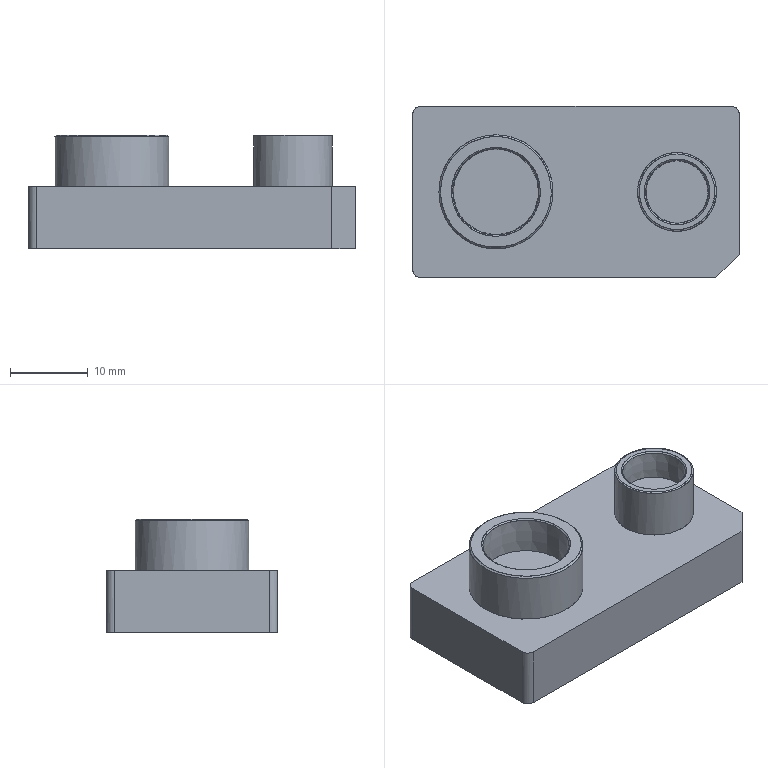NC program | PowerMill | posted by the shop | part box 42 x 22 x 14.621 mm
Lines 4390 to 5888 of 126517:
( TOOL ID   D4C_1_1 )
( TOOL DIA. 4. TIP RAD 0 LENGTH 61.8 )
( Z = -6.75 )
T2 M6
T3
G91 G28 Z0
G0 G90 G54
M08
S18000 M3
X0 Y0 M8
G43 Z9.801 H2
X-19.073 Y-5.404
Z.797
G1 Z-.403 F3600
X-19.051 Y-5.405 F6000
G3 X-18.846 Y-5.215 I.008 J.198
G1 X-18.79 Y-3.832
X-19.034 Y-3.291
X-19.237 Y-2.684
X-19.48 Y-1.708
X-19.605 Y-.732
X-19.627 Y.244
X-19.557 Y1.22
X-19.373 Y2.196
X-19.034 Y3.291
X-18.546 Y4.373
X-18.058 Y5.183
X-17.756 Y5.613
X-17.082 Y6.417
X-16.594 Y6.892
X-15.772 Y7.565
X-15.13 Y7.982
X-14.642 Y8.259
X-14.154 Y8.499
X-13.665 Y8.706
X-13.177 Y8.88
X-12.689 Y9.023
X-11.713 Y9.218
X-10.737 Y9.319
X-9.761 Y9.318
X-8.785 Y9.201
X-7.94 Y9.029
X-7.321 Y8.842
X-6.833 Y8.664
X-6.345 Y8.452
X-5.601 Y8.053
X-4.837 Y7.565
X-4.392 Y7.222
X-3.904 Y6.794
X-3.416 Y6.294
X-2.853 Y5.613
X-2.44 Y5.027
X-1.952 Y4.152
X-1.727 Y3.66
X-1.464 Y2.987
X-1.372 Y2.684
X-1.129 Y1.708
X-1.004 Y.732
X-.982 Y-.244
X-1.051 Y-1.22
X-1.236 Y-2.196
X-1.464 Y-2.987
X-1.727 Y-3.66
X-1.95 Y-4.148
X-2.44 Y-5.027
X-2.853 Y-5.613
X-3.249 Y-6.101
X-3.904 Y-6.794
X-4.392 Y-7.222
X-4.837 Y-7.565
X-5.369 Y-7.921
X-5.857 Y-8.205
X-6.561 Y-8.541
X-7.321 Y-8.842
X-7.94 Y-9.029
X-8.785 Y-9.201
X-9.761 Y-9.318
X-10.737 Y-9.319
X-11.713 Y-9.218
X-12.668 Y-9.029
X-13.177 Y-8.88
X-14.048 Y-8.541
X-14.642 Y-8.259
X-15.13 Y-7.982
X-15.772 Y-7.565
X-16.382 Y-7.077
X-17.082 Y-6.417
X-17.57 Y-5.855
X-18.1 Y-5.125
X-18.546 Y-4.373
X-18.79 Y-3.832
X-19.073 Y-5.408 Z-.596
X-19.051 Y-5.409
G3 X-18.846 Y-5.219 I.008 J.198
G1 X-18.79 Y-3.832
X-19.034 Y-3.291
X-19.237 Y-2.684
X-19.48 Y-1.708
X-19.605 Y-.732
X-19.627 Y.244
X-19.557 Y1.22
X-19.373 Y2.196
X-19.034 Y3.291
X-18.546 Y4.373
X-18.058 Y5.183
X-17.756 Y5.613
X-17.082 Y6.417
X-16.594 Y6.892
X-15.772 Y7.565
X-15.13 Y7.982
X-14.642 Y8.259
X-14.154 Y8.499
X-13.665 Y8.706
X-13.177 Y8.88
X-12.689 Y9.023
X-11.713 Y9.218
X-10.737 Y9.319
X-9.761 Y9.318
X-8.785 Y9.201
X-7.94 Y9.029
X-7.321 Y8.842
X-6.833 Y8.664
X-6.345 Y8.452
X-5.601 Y8.053
X-4.837 Y7.565
X-4.392 Y7.222
X-3.904 Y6.794
X-3.416 Y6.294
X-2.853 Y5.613
X-2.44 Y5.027
X-1.952 Y4.152
X-1.727 Y3.66
X-1.464 Y2.987
X-1.372 Y2.684
X-1.129 Y1.708
X-1.004 Y.732
X-.982 Y-.244
X-1.051 Y-1.22
X-1.236 Y-2.196
X-1.464 Y-2.987
X-1.727 Y-3.66
X-1.95 Y-4.148
X-2.44 Y-5.027
X-2.853 Y-5.613
X-3.249 Y-6.101
X-3.904 Y-6.794
X-4.392 Y-7.222
X-4.837 Y-7.565
X-5.369 Y-7.921
X-5.857 Y-8.205
X-6.561 Y-8.541
X-7.321 Y-8.842
X-7.94 Y-9.029
X-8.785 Y-9.201
X-9.761 Y-9.318
X-10.737 Y-9.319
X-11.713 Y-9.218
X-12.668 Y-9.029
X-13.177 Y-8.88
X-14.048 Y-8.541
X-14.642 Y-8.259
X-15.13 Y-7.982
X-15.772 Y-7.565
X-16.382 Y-7.077
X-17.082 Y-6.417
X-17.57 Y-5.855
X-18.1 Y-5.125
X-18.546 Y-4.373
X-18.79 Y-3.832
X-19.073 Y-5.408 Z-.79
X-19.051 Y-5.409
G3 X-18.846 Y-5.219 I.008 J.198
G1 X-18.79 Y-3.832
X-19.034 Y-3.291
X-19.237 Y-2.684
X-19.48 Y-1.708
X-19.605 Y-.732
X-19.627 Y.244
X-19.557 Y1.22
X-19.373 Y2.196
X-19.034 Y3.291
X-18.546 Y4.373
X-18.058 Y5.183
X-17.756 Y5.613
X-17.082 Y6.417
X-16.594 Y6.892
X-15.772 Y7.565
X-15.13 Y7.982
X-14.642 Y8.259
X-14.154 Y8.499
X-13.665 Y8.706
X-13.177 Y8.88
X-12.689 Y9.023
X-11.713 Y9.218
X-10.737 Y9.319
X-9.761 Y9.318
X-8.785 Y9.201
X-7.94 Y9.029
X-7.321 Y8.842
X-6.833 Y8.664
X-6.345 Y8.452
X-5.601 Y8.053
X-4.837 Y7.565
X-4.392 Y7.222
X-3.904 Y6.794
X-3.416 Y6.294
X-2.853 Y5.613
X-2.44 Y5.027
X-2.129 Y4.468
X-1.952 Y4.152
X-1.95 Y4.148
X-1.727 Y3.66
X-1.464 Y2.987
X-1.372 Y2.684
X-1.129 Y1.708
X-1.004 Y.732
X-.982 Y-.244
X-1.051 Y-1.22
X-1.236 Y-2.196
X-1.464 Y-2.987
X-1.727 Y-3.66
X-1.779 Y-3.773
X-1.95 Y-4.148
X-1.952 Y-4.15
Y-4.152
X-2.44 Y-5.027
X-2.853 Y-5.613
X-3.249 Y-6.101
X-3.904 Y-6.794
X-4.392 Y-7.222
X-4.837 Y-7.565
X-5.369 Y-7.921
X-5.857 Y-8.205
X-6.561 Y-8.541
X-7.321 Y-8.842
X-7.94 Y-9.029
X-8.785 Y-9.201
X-9.761 Y-9.318
X-10.737 Y-9.319
X-11.713 Y-9.218
X-12.668 Y-9.029
X-13.177 Y-8.88
X-14.048 Y-8.541
X-14.642 Y-8.259
X-15.13 Y-7.982
X-15.772 Y-7.565
X-16.382 Y-7.077
X-17.082 Y-6.417
X-17.57 Y-5.855
X-18.1 Y-5.125
X-18.546 Y-4.373
X-18.79 Y-3.832
X-19.073 Y-5.408 Z-.984
X-19.051 Y-5.409
G3 X-18.846 Y-5.219 I.008 J.198
G1 X-18.79 Y-3.832
X-19.034 Y-3.291
X-19.237 Y-2.684
X-19.48 Y-1.708
X-19.605 Y-.732
X-19.627 Y.244
X-19.558 Y1.22
X-19.373 Y2.196
X-19.034 Y3.291
X-18.546 Y4.373
X-18.058 Y5.183
X-17.756 Y5.613
X-17.082 Y6.417
X-16.594 Y6.892
X-15.772 Y7.565
X-15.13 Y7.982
X-14.642 Y8.259
X-14.154 Y8.499
X-13.665 Y8.706
X-13.177 Y8.88
X-12.689 Y9.023
X-11.713 Y9.218
X-10.737 Y9.319
X-9.761 Y9.318
X-8.785 Y9.201
X-7.94 Y9.029
X-7.321 Y8.842
X-6.833 Y8.664
X-6.345 Y8.452
X-5.601 Y8.053
X-4.837 Y7.565
X-4.392 Y7.222
X-3.904 Y6.794
X-3.416 Y6.294
X-2.853 Y5.613
X-2.44 Y5.027
X-1.95 Y4.148
X-1.727 Y3.66
X-1.464 Y2.987
X-1.372 Y2.684
X-1.129 Y1.708
X-1.004 Y.732
X-.982 Y-.244
X-1.051 Y-1.22
X-1.236 Y-2.196
X-1.464 Y-2.987
X-1.727 Y-3.66
X-1.83 Y-3.884
X-1.95 Y-4.148
X-1.951 Y-4.15
X-1.952 Y-4.152
X-2.44 Y-5.027
X-2.853 Y-5.613
X-3.249 Y-6.101
X-3.904 Y-6.794
X-4.392 Y-7.222
X-4.837 Y-7.565
X-5.369 Y-7.921
X-5.857 Y-8.205
X-6.561 Y-8.541
X-7.321 Y-8.842
X-7.94 Y-9.029
X-8.785 Y-9.201
X-9.761 Y-9.318
X-10.737 Y-9.319
X-11.713 Y-9.218
X-12.668 Y-9.029
X-13.177 Y-8.88
X-14.048 Y-8.541
X-14.642 Y-8.259
X-15.13 Y-7.982
X-15.772 Y-7.565
X-16.382 Y-7.077
X-17.082 Y-6.417
X-17.57 Y-5.855
X-18.1 Y-5.125
X-18.546 Y-4.373
X-18.79 Y-3.832
X-19.073 Y-5.408 Z-1.177
X-19.051 Y-5.409
G3 X-18.846 Y-5.219 I.008 J.198
G1 X-18.79 Y-3.832
X-19.034 Y-3.291
X-19.237 Y-2.684
X-19.48 Y-1.708
X-19.605 Y-.732
X-19.627 Y.244
X-19.558 Y1.22
X-19.373 Y2.196
X-19.034 Y3.291
X-18.546 Y4.373
X-18.058 Y5.183
X-17.756 Y5.613
X-17.082 Y6.417
X-16.594 Y6.892
X-15.772 Y7.565
X-15.13 Y7.982
X-14.642 Y8.259
X-14.154 Y8.499
X-13.665 Y8.706
X-13.177 Y8.88
X-12.689 Y9.023
X-11.713 Y9.218
X-10.737 Y9.319
X-9.761 Y9.318
X-8.785 Y9.201
X-7.94 Y9.029
X-7.321 Y8.842
X-6.833 Y8.664
X-6.345 Y8.452
X-5.601 Y8.053
X-4.837 Y7.565
X-4.392 Y7.222
X-3.904 Y6.794
X-3.416 Y6.294
X-2.853 Y5.613
X-2.44 Y5.027
X-1.95 Y4.148
X-1.727 Y3.66
X-1.464 Y2.987
X-1.372 Y2.684
X-1.129 Y1.708
X-1.004 Y.732
X-.982 Y-.244
X-1.051 Y-1.22
X-1.236 Y-2.196
X-1.464 Y-2.987
X-1.727 Y-3.66
X-1.88 Y-3.993
X-1.951 Y-4.148
Y-4.15
X-1.952 Y-4.152
X-2.44 Y-5.027
X-2.853 Y-5.613
X-3.249 Y-6.101
X-3.904 Y-6.794
X-4.392 Y-7.222
X-4.837 Y-7.565
X-5.369 Y-7.921
X-5.857 Y-8.205
X-6.561 Y-8.541
X-7.321 Y-8.842
X-7.94 Y-9.029
X-8.785 Y-9.201
X-9.761 Y-9.318
X-10.737 Y-9.319
X-11.713 Y-9.218
X-12.668 Y-9.029
X-13.177 Y-8.88
X-14.048 Y-8.541
X-14.642 Y-8.259
X-15.13 Y-7.982
X-15.772 Y-7.565
X-16.382 Y-7.077
X-17.082 Y-6.417
X-17.57 Y-5.855
X-18.1 Y-5.125
X-18.546 Y-4.373
X-18.79 Y-3.832
X-19.073 Y-5.408 Z-1.371
X-19.051 Y-5.409
G3 X-18.846 Y-5.219 I.008 J.198
G1 X-18.79 Y-3.832
X-19.034 Y-3.291
X-19.237 Y-2.684
X-19.48 Y-1.708
X-19.605 Y-.732
X-19.627 Y.244
X-19.558 Y1.22
X-19.373 Y2.196
X-19.034 Y3.291
X-18.546 Y4.373
X-18.058 Y5.183
X-17.756 Y5.613
X-17.082 Y6.417
X-16.594 Y6.892
X-15.772 Y7.565
X-15.13 Y7.982
X-14.642 Y8.259
X-14.154 Y8.499
X-13.665 Y8.706
X-13.177 Y8.88
X-12.689 Y9.023
X-11.713 Y9.218
X-10.737 Y9.319
X-9.761 Y9.318
X-8.785 Y9.201
X-7.94 Y9.029
X-7.321 Y8.842
X-6.833 Y8.664
X-6.345 Y8.452
X-5.601 Y8.053
X-4.837 Y7.565
X-4.392 Y7.222
X-3.904 Y6.794
X-3.416 Y6.294
X-2.853 Y5.613
X-2.44 Y5.027
X-1.95 Y4.148
X-1.727 Y3.66
X-1.464 Y2.987
X-1.372 Y2.684
X-1.129 Y1.708
X-1.004 Y.732
X-.982 Y-.244
X-1.051 Y-1.22
X-1.236 Y-2.196
X-1.464 Y-2.987
X-1.727 Y-3.66
X-1.929 Y-4.101
X-1.951 Y-4.148
Y-4.149
X-1.952 Y-4.152
X-2.44 Y-5.027
X-2.853 Y-5.613
X-3.249 Y-6.101
X-3.904 Y-6.794
X-4.392 Y-7.222
X-4.837 Y-7.565
X-5.369 Y-7.921
X-5.857 Y-8.205
X-6.561 Y-8.541
X-7.321 Y-8.842
X-7.94 Y-9.029
X-8.785 Y-9.201
X-9.761 Y-9.318
X-10.737 Y-9.319
X-11.713 Y-9.218
X-12.668 Y-9.029
X-13.177 Y-8.88
X-14.048 Y-8.541
X-14.642 Y-8.259
X-15.13 Y-7.982
X-15.772 Y-7.565
X-16.382 Y-7.077
X-17.082 Y-6.417
X-17.57 Y-5.855
X-18.1 Y-5.125
X-18.546 Y-4.373
X-18.79 Y-3.832
X-19.073 Y-5.408 Z-1.565
X-19.051 Y-5.409
G3 X-18.846 Y-5.219 I.008 J.198
G1 X-18.79 Y-3.832
X-19.034 Y-3.291
X-19.237 Y-2.684
X-19.48 Y-1.708
X-19.605 Y-.732
X-19.627 Y.244
X-19.558 Y1.22
X-19.373 Y2.196
X-19.034 Y3.291
X-18.546 Y4.373
X-18.058 Y5.183
X-17.756 Y5.613
X-17.082 Y6.417
X-16.594 Y6.892
X-15.772 Y7.565
X-15.13 Y7.982
X-14.642 Y8.259
X-14.154 Y8.499
X-13.665 Y8.706
X-13.177 Y8.88
X-12.689 Y9.023
X-11.713 Y9.218
X-10.737 Y9.319
X-9.761 Y9.318
X-8.785 Y9.201
X-7.94 Y9.029
X-7.321 Y8.842
X-6.833 Y8.664
X-6.345 Y8.452
X-5.601 Y8.053
X-4.837 Y7.565
X-4.392 Y7.222
X-3.904 Y6.794
X-3.416 Y6.294
X-2.853 Y5.613
X-2.44 Y5.027
X-1.95 Y4.148
X-1.727 Y3.66
X-1.464 Y2.987
X-1.372 Y2.684
X-1.129 Y1.708
X-1.004 Y.732
X-.982 Y-.244
X-1.051 Y-1.22
X-1.236 Y-2.196
X-1.464 Y-2.987
X-1.727 Y-3.66
X-1.952 Y-4.152
X-2.44 Y-5.027
X-2.853 Y-5.613
X-3.249 Y-6.101
X-3.904 Y-6.794
X-4.392 Y-7.222
X-4.837 Y-7.565
X-5.369 Y-7.921
X-5.857 Y-8.205
X-6.561 Y-8.541
X-7.321 Y-8.842
X-7.94 Y-9.029
X-8.785 Y-9.201
X-9.761 Y-9.318
X-10.737 Y-9.319
X-11.713 Y-9.218
X-12.668 Y-9.029
X-13.177 Y-8.88
X-14.048 Y-8.541
X-14.642 Y-8.259
X-15.13 Y-7.982
X-15.772 Y-7.565
X-16.382 Y-7.077
X-17.082 Y-6.417
X-17.57 Y-5.855
X-18.1 Y-5.125
X-18.546 Y-4.373
X-18.79 Y-3.832
X-19.073 Y-5.408 Z-1.758
X-19.051 Y-5.409
G3 X-18.846 Y-5.219 I.008 J.198
G1 X-18.79 Y-3.832
X-19.034 Y-3.291
X-19.237 Y-2.684
X-19.48 Y-1.708
X-19.605 Y-.732
X-19.627 Y.244
X-19.558 Y1.22
X-19.373 Y2.196
X-19.034 Y3.291
X-18.546 Y4.373
X-18.058 Y5.183
X-17.756 Y5.613
X-17.082 Y6.417
X-16.594 Y6.892
X-15.772 Y7.565
X-15.13 Y7.982
X-14.642 Y8.259
X-14.154 Y8.499
X-13.665 Y8.706
X-13.177 Y8.88
X-12.689 Y9.023
X-11.713 Y9.218
X-10.737 Y9.319
X-9.761 Y9.318
X-8.785 Y9.201
X-7.94 Y9.029
X-7.321 Y8.842
X-6.833 Y8.664
X-6.345 Y8.452
X-5.601 Y8.053
X-4.837 Y7.565
X-4.392 Y7.222
X-3.904 Y6.794
X-3.416 Y6.294
X-2.853 Y5.613
X-2.44 Y5.027
X-1.95 Y4.148
X-1.727 Y3.66
X-1.464 Y2.987
X-1.372 Y2.684
X-1.129 Y1.708
X-1.004 Y.732
X-.982 Y-.244
X-1.051 Y-1.22
X-1.236 Y-2.196
X-1.464 Y-2.987
X-1.727 Y-3.66
X-1.952 Y-4.152
X-2.44 Y-5.027
X-2.853 Y-5.613
X-3.249 Y-6.101
X-3.904 Y-6.794
X-4.392 Y-7.222
X-4.837 Y-7.565
X-5.369 Y-7.921
X-5.857 Y-8.205
X-6.561 Y-8.541
X-7.321 Y-8.842
X-7.94 Y-9.029
X-8.785 Y-9.201
X-9.761 Y-9.318
X-10.737 Y-9.319
X-11.713 Y-9.218
X-12.668 Y-9.029
X-13.177 Y-8.88
X-14.048 Y-8.541
X-14.642 Y-8.259
X-15.13 Y-7.982
X-15.772 Y-7.565
X-16.382 Y-7.077
X-17.082 Y-6.417
X-17.57 Y-5.855
X-18.1 Y-5.125
X-18.546 Y-4.373
X-18.79 Y-3.832
X-19.073 Y-5.408 Z-1.952
X-19.051 Y-5.409
G3 X-18.846 Y-5.219 I.008 J.198
G1 X-18.79 Y-3.832
X-19.034 Y-3.291
X-19.237 Y-2.684
X-19.48 Y-1.708
X-19.605 Y-.732
X-19.627 Y.244
X-19.558 Y1.22
X-19.373 Y2.196
X-19.034 Y3.291
X-18.546 Y4.373
X-18.058 Y5.183
X-17.756 Y5.613
X-17.082 Y6.417
X-16.594 Y6.892
X-15.772 Y7.565
X-15.13 Y7.982
X-14.642 Y8.259
X-14.154 Y8.499
X-13.665 Y8.706
X-13.177 Y8.88
X-12.689 Y9.023
X-11.713 Y9.218
X-10.737 Y9.319
X-9.761 Y9.318
X-8.785 Y9.201
X-7.94 Y9.029
X-7.321 Y8.842
X-6.833 Y8.664
X-6.345 Y8.452
X-5.601 Y8.053
X-4.837 Y7.565
X-4.392 Y7.222
X-3.904 Y6.794
X-3.416 Y6.294
X-2.853 Y5.613
X-2.44 Y5.027
X-1.95 Y4.148
X-1.727 Y3.66
X-1.464 Y2.988
X-1.372 Y2.684
X-1.129 Y1.708
X-1.004 Y.732
X-.982 Y-.244
X-1.051 Y-1.22
X-1.236 Y-2.196
X-1.464 Y-2.988
X-1.727 Y-3.66
X-1.952 Y-4.152
X-2.44 Y-5.027
X-2.853 Y-5.613
X-3.249 Y-6.101
X-3.904 Y-6.794
X-4.392 Y-7.222
X-4.837 Y-7.565
X-5.369 Y-7.921
X-5.857 Y-8.205
X-6.561 Y-8.541
X-7.321 Y-8.842
X-7.94 Y-9.029
X-8.785 Y-9.201
X-9.761 Y-9.318
X-10.737 Y-9.319
X-11.713 Y-9.218
X-12.668 Y-9.029
X-13.177 Y-8.88
X-14.048 Y-8.541
X-14.642 Y-8.259
X-15.13 Y-7.982
X-15.772 Y-7.565
X-16.382 Y-7.077
X-17.082 Y-6.417
X-17.57 Y-5.855
X-18.1 Y-5.125
X-18.546 Y-4.373
X-18.79 Y-3.832
X-19.073 Y-5.408 Z-2.146
X-19.051 Y-5.409
G3 X-18.846 Y-5.219 I.008 J.198
G1 X-18.79 Y-3.832
X-19.034 Y-3.291
X-19.237 Y-2.684
X-19.48 Y-1.708
X-19.605 Y-.732
X-19.627 Y.244
X-19.558 Y1.22
X-19.373 Y2.196
X-19.034 Y3.291
X-18.546 Y4.373
X-18.058 Y5.183
X-17.756 Y5.613
X-17.082 Y6.417
X-16.594 Y6.892
X-15.772 Y7.565
X-15.13 Y7.982
X-14.642 Y8.259
X-14.154 Y8.499
X-13.665 Y8.706
X-13.177 Y8.88
X-12.689 Y9.023
X-11.713 Y9.219
X-10.737 Y9.319
X-9.761 Y9.318
X-8.785 Y9.201
X-7.94 Y9.029
X-7.321 Y8.842
X-6.833 Y8.664
X-6.345 Y8.452
X-5.601 Y8.053
X-4.837 Y7.565
X-4.392 Y7.222
X-3.904 Y6.794
X-3.416 Y6.294
X-2.853 Y5.613
X-2.44 Y5.027
X-1.95 Y4.148
X-1.727 Y3.66
X-1.464 Y2.988
X-1.372 Y2.684
X-1.129 Y1.708
X-1.004 Y.732
X-.982 Y-.244
X-1.051 Y-1.22
X-1.236 Y-2.196
X-1.464 Y-2.988
X-1.727 Y-3.66
X-1.952 Y-4.152
X-2.44 Y-5.027
X-2.853 Y-5.613
X-3.249 Y-6.101
X-3.904 Y-6.794
X-4.392 Y-7.222
X-4.837 Y-7.565
X-5.369 Y-7.921
X-5.857 Y-8.205
X-6.561 Y-8.541
X-7.321 Y-8.842
X-7.94 Y-9.029
X-8.785 Y-9.201
X-9.761 Y-9.318
X-10.737 Y-9.319
X-11.713 Y-9.219
X-12.668 Y-9.029
X-13.177 Y-8.88
X-14.048 Y-8.541
X-14.642 Y-8.259
X-15.13 Y-7.982
X-15.772 Y-7.565
X-16.382 Y-7.077
X-17.082 Y-6.417
X-17.57 Y-5.855
X-18.1 Y-5.125
X-18.546 Y-4.373
X-18.79 Y-3.832
X-19.073 Y-5.408 Z-2.339
X-19.051 Y-5.409
G3 X-18.846 Y-5.219 I.008 J.198
G1 X-18.79 Y-3.832
X-19.034 Y-3.291
X-19.237 Y-2.684
X-19.48 Y-1.708
X-19.605 Y-.732
X-19.627 Y.244
X-19.558 Y1.22
X-19.373 Y2.196
X-19.034 Y3.291
X-18.546 Y4.373
X-18.058 Y5.183
X-17.756 Y5.613
X-17.082 Y6.417
X-16.594 Y6.892
X-15.772 Y7.565
X-15.13 Y7.982
X-14.642 Y8.259
X-14.154 Y8.499
X-13.665 Y8.706
X-13.177 Y8.88
X-12.689 Y9.023
X-11.713 Y9.219
X-10.737 Y9.319
X-9.761 Y9.318
X-8.785 Y9.201
X-7.94 Y9.029
X-7.321 Y8.842
X-6.833 Y8.664
X-6.345 Y8.452
X-5.601 Y8.053
X-4.837 Y7.565
X-4.392 Y7.222
X-3.904 Y6.794
X-3.416 Y6.294
X-2.853 Y5.613
X-2.44 Y5.027
X-1.95 Y4.148
X-1.727 Y3.66
X-1.464 Y2.988
X-1.372 Y2.684
X-1.129 Y1.708
X-1.004 Y.732
X-.982 Y-.244
X-1.051 Y-1.22
X-1.236 Y-2.196
X-1.464 Y-2.988
X-1.727 Y-3.66
X-1.952 Y-4.152
X-2.44 Y-5.027
X-2.853 Y-5.613
X-3.249 Y-6.101
X-3.904 Y-6.794
X-4.392 Y-7.222
X-4.837 Y-7.565
X-5.369 Y-7.921
X-5.857 Y-8.205
X-6.561 Y-8.541
X-7.321 Y-8.842
X-7.94 Y-9.029
X-8.785 Y-9.201
X-9.761 Y-9.318
X-10.737 Y-9.319
X-11.713 Y-9.219
X-12.669 Y-9.029
X-13.177 Y-8.88
X-14.048 Y-8.541
X-14.642 Y-8.259
X-15.13 Y-7.982
X-15.772 Y-7.565
X-16.382 Y-7.077
X-17.082 Y-6.417
X-17.57 Y-5.855
X-18.1 Y-5.125
X-18.546 Y-4.373
X-18.79 Y-3.832
X-19.073 Y-5.408 Z-2.533
X-19.051 Y-5.409
G3 X-18.846 Y-5.219 I.008 J.198
G1 X-18.79 Y-3.832
X-19.034 Y-3.291
X-19.237 Y-2.684
X-19.48 Y-1.708
X-19.605 Y-.732
X-19.627 Y.244
X-19.558 Y1.22
X-19.373 Y2.196
X-19.034 Y3.291
X-18.546 Y4.373
X-18.058 Y5.183
X-17.756 Y5.613
X-17.082 Y6.417
X-16.594 Y6.892
X-15.772 Y7.565
X-15.13 Y7.982
X-14.642 Y8.259
X-14.154 Y8.499
X-13.665 Y8.706
X-13.177 Y8.88
X-12.689 Y9.023
X-11.713 Y9.219
X-10.737 Y9.319
X-9.761 Y9.318
X-8.785 Y9.201
X-7.94 Y9.029
X-7.321 Y8.842
X-6.833 Y8.664
X-6.345 Y8.452
X-5.601 Y8.053
X-4.837 Y7.565
X-4.392 Y7.222
X-3.904 Y6.794
X-3.416 Y6.294
X-2.853 Y5.613
X-2.44 Y5.027
X-1.95 Y4.148
X-1.727 Y3.66
X-1.464 Y2.988
X-1.372 Y2.684
X-1.129 Y1.708
X-1.004 Y.732
X-.982 Y-.244
X-1.051 Y-1.22
X-1.236 Y-2.196
X-1.464 Y-2.988
X-1.727 Y-3.66
X-1.952 Y-4.152
X-2.44 Y-5.027
X-2.853 Y-5.613
X-3.249 Y-6.101
X-3.904 Y-6.794
X-4.392 Y-7.222
X-4.837 Y-7.565
X-5.369 Y-7.921
X-5.857 Y-8.205
X-6.561 Y-8.541
X-7.321 Y-8.842
X-7.94 Y-9.029
X-8.785 Y-9.201
X-9.761 Y-9.318
X-10.737 Y-9.319
X-11.713 Y-9.219
X-12.669 Y-9.029
X-13.177 Y-8.88
X-14.048 Y-8.541
X-14.642 Y-8.259
X-15.13 Y-7.982
X-15.772 Y-7.565
X-16.382 Y-7.077
X-17.082 Y-6.417
X-17.57 Y-5.855
X-18.1 Y-5.125
X-18.546 Y-4.373
X-18.79 Y-3.832
X-19.073 Y-5.408 Z-2.727
X-19.051 Y-5.409
G3 X-18.846 Y-5.219 I.008 J.198
G1 X-18.79 Y-3.832
X-19.034 Y-3.291
X-19.237 Y-2.684
X-19.48 Y-1.708
X-19.605 Y-.732
X-19.627 Y.244
X-19.558 Y1.22
X-19.373 Y2.196
X-19.034 Y3.291
X-18.546 Y4.373
X-18.058 Y5.183
X-17.756 Y5.613
X-17.082 Y6.417
X-16.594 Y6.892
X-15.772 Y7.565
X-15.13 Y7.982
X-14.642 Y8.259
X-14.154 Y8.499
X-13.665 Y8.706
X-13.177 Y8.88
X-12.689 Y9.023
X-11.713 Y9.219
X-10.737 Y9.319
X-9.761 Y9.318
X-8.785 Y9.201
X-7.94 Y9.029
X-7.321 Y8.842
X-6.833 Y8.664
X-6.345 Y8.452
X-5.601 Y8.053
X-4.837 Y7.565
X-4.392 Y7.222
X-3.904 Y6.794
X-3.416 Y6.294
X-2.853 Y5.613
X-2.44 Y5.027
X-1.95 Y4.148
X-1.727 Y3.66
X-1.464 Y2.988
X-1.372 Y2.684
X-1.129 Y1.708
X-1.004 Y.732
X-.982 Y-.244
X-1.051 Y-1.22
X-1.236 Y-2.196
X-1.464 Y-2.988
X-1.727 Y-3.66
X-1.952 Y-4.152
X-2.44 Y-5.027
X-2.853 Y-5.613
X-3.249 Y-6.101
X-3.904 Y-6.794
X-4.392 Y-7.222
X-4.837 Y-7.565
X-5.369 Y-7.921
X-5.857 Y-8.205
X-6.561 Y-8.541
X-7.321 Y-8.842
X-7.94 Y-9.029
X-8.785 Y-9.201
X-9.761 Y-9.318
X-10.737 Y-9.319
X-11.713 Y-9.219
X-12.669 Y-9.029
X-13.177 Y-8.88
X-14.048 Y-8.541
X-14.642 Y-8.259
X-15.13 Y-7.982
X-15.772 Y-7.565
X-16.382 Y-7.077
X-17.082 Y-6.417
X-17.57 Y-5.855
X-18.1 Y-5.125
X-18.546 Y-4.373
X-18.79 Y-3.832
X-19.073 Y-5.408 Z-2.92
X-19.051 Y-5.409
G3 X-18.846 Y-5.219 I.008 J.198
G1 X-18.79 Y-3.832
X-19.034 Y-3.291
X-19.237 Y-2.684
X-19.48 Y-1.708
X-19.605 Y-.732
X-19.627 Y.244
X-19.558 Y1.22
X-19.373 Y2.196
X-19.034 Y3.291
X-18.546 Y4.373
X-18.058 Y5.183
X-17.756 Y5.613
X-17.082 Y6.417
X-16.594 Y6.892
X-15.772 Y7.565
X-15.13 Y7.982
X-14.642 Y8.259
X-14.154 Y8.499
X-13.665 Y8.706
X-13.177 Y8.88
X-12.689 Y9.023
X-11.713 Y9.219
X-10.737 Y9.319
X-9.761 Y9.318
X-8.785 Y9.201
X-7.94 Y9.029
X-7.321 Y8.842
X-6.833 Y8.664
X-6.345 Y8.452
X-5.601 Y8.053
X-4.837 Y7.565
X-4.392 Y7.222
X-3.904 Y6.794
X-3.416 Y6.294
X-2.853 Y5.613
X-2.44 Y5.027
X-1.95 Y4.148
X-1.727 Y3.66
X-1.464 Y2.988
X-1.372 Y2.684
X-1.129 Y1.708
X-1.004 Y.732
X-.982 Y-.244
X-1.051 Y-1.22
X-1.236 Y-2.196
X-1.464 Y-2.988
X-1.727 Y-3.66
X-1.952 Y-4.152
X-2.44 Y-5.027
X-2.853 Y-5.613
X-3.249 Y-6.101
X-3.904 Y-6.794
X-4.392 Y-7.222
X-4.837 Y-7.565
X-5.369 Y-7.921
X-5.857 Y-8.205
X-6.561 Y-8.541
X-7.321 Y-8.842
X-7.94 Y-9.029
X-8.785 Y-9.201
X-9.761 Y-9.318
X-10.737 Y-9.319
X-11.713 Y-9.219
X-12.669 Y-9.029
X-13.177 Y-8.88
X-14.048 Y-8.541
X-14.642 Y-8.259
X-15.13 Y-7.982
X-15.772 Y-7.565
X-16.382 Y-7.077
X-17.082 Y-6.417
X-17.57 Y-5.855
X-18.1 Y-5.125
X-18.546 Y-4.373
X-18.79 Y-3.832
X-19.073 Y-5.408 Z-3.114
X-19.051 Y-5.409
G3 X-18.846 Y-5.219 I.008 J.198
G1 X-18.79 Y-3.832
X-19.034 Y-3.291
X-19.237 Y-2.684
X-19.48 Y-1.708
X-19.605 Y-.732
X-19.627 Y.244
X-19.558 Y1.22
X-19.373 Y2.196
X-19.034 Y3.291
X-18.546 Y4.373
X-18.058 Y5.183
X-17.756 Y5.613
X-17.082 Y6.417
X-16.594 Y6.892
X-15.772 Y7.565
X-15.13 Y7.982
X-14.642 Y8.259
X-14.154 Y8.499
X-13.665 Y8.706
X-13.177 Y8.88
X-12.689 Y9.023
X-11.713 Y9.219
X-10.737 Y9.319
X-9.761 Y9.318
X-8.785 Y9.201
X-7.94 Y9.029
X-7.321 Y8.842
X-6.833 Y8.664
X-6.345 Y8.452
X-5.601 Y8.053
X-4.837 Y7.565
X-4.392 Y7.222
X-3.904 Y6.794
X-3.416 Y6.294
X-2.853 Y5.613
X-2.44 Y5.027
X-1.95 Y4.148
X-1.727 Y3.66
X-1.464 Y2.988
X-1.372 Y2.684
X-1.129 Y1.708
X-1.004 Y.732
X-.982 Y-.244
X-1.051 Y-1.22
X-1.236 Y-2.196
X-1.464 Y-2.988
X-1.727 Y-3.66
X-1.952 Y-4.152
X-2.44 Y-5.027
X-2.853 Y-5.613
X-3.249 Y-6.101
X-3.904 Y-6.794
X-4.392 Y-7.222
X-4.837 Y-7.565
X-5.369 Y-7.921
X-5.857 Y-8.205
X-6.561 Y-8.541
X-7.321 Y-8.842
X-7.94 Y-9.029
X-8.785 Y-9.201
X-9.761 Y-9.318
X-10.737 Y-9.319
X-11.713 Y-9.219
X-12.669 Y-9.029
X-13.177 Y-8.88
X-14.048 Y-8.541
X-14.642 Y-8.259
X-15.13 Y-7.982
X-15.772 Y-7.565
X-16.382 Y-7.077
X-17.082 Y-6.417
X-17.57 Y-5.855
X-18.1 Y-5.125
X-18.546 Y-4.373
X-18.79 Y-3.832
X-19.073 Y-5.408 Z-3.308
X-19.051 Y-5.409
G3 X-18.846 Y-5.219 I.008 J.198
G1 X-18.79 Y-3.832
X-19.034 Y-3.291
X-19.237 Y-2.684
X-19.48 Y-1.708
X-19.605 Y-.732
X-19.627 Y.244
X-19.558 Y1.22
X-19.373 Y2.196
X-19.034 Y3.291
X-18.546 Y4.373
X-18.058 Y5.183
X-17.756 Y5.613
X-17.082 Y6.417
X-16.594 Y6.892
X-15.772 Y7.565
X-15.13 Y7.982
X-14.642 Y8.259
X-14.154 Y8.499
X-13.665 Y8.706
X-13.177 Y8.88
X-12.689 Y9.023
X-11.713 Y9.219
X-10.737 Y9.319
X-9.761 Y9.318
X-8.785 Y9.201
X-7.94 Y9.029
X-7.321 Y8.842
X-6.833 Y8.664
X-6.345 Y8.452
X-5.601 Y8.053
X-4.837 Y7.565
X-4.392 Y7.222
X-3.904 Y6.794
X-3.416 Y6.294
X-2.853 Y5.613
X-2.44 Y5.027
X-1.95 Y4.148
X-1.727 Y3.66
X-1.464 Y2.988
X-1.372 Y2.684
X-1.129 Y1.708
X-1.004 Y.732
X-.982 Y-.244
X-1.051 Y-1.22
X-1.236 Y-2.196
X-1.464 Y-2.988
X-1.727 Y-3.66
X-1.952 Y-4.152
X-2.44 Y-5.027
X-2.853 Y-5.613
X-3.249 Y-6.101
X-3.904 Y-6.794
X-4.392 Y-7.222
X-4.837 Y-7.565
X-5.369 Y-7.921
X-5.857 Y-8.205
X-6.561 Y-8.541
X-7.321 Y-8.842
X-7.94 Y-9.029
X-8.785 Y-9.201
X-9.761 Y-9.318
X-10.737 Y-9.319
X-11.713 Y-9.219
X-12.669 Y-9.029
X-13.177 Y-8.88
X-14.048 Y-8.541
X-14.642 Y-8.259
X-15.13 Y-7.982
X-15.772 Y-7.565
X-16.382 Y-7.077
X-17.082 Y-6.417
X-17.57 Y-5.855
X-18.1 Y-5.125
X-18.546 Y-4.373
X-18.79 Y-3.832
X-19.073 Y-5.408 Z-3.501
X-19.051 Y-5.409
G3 X-18.846 Y-5.219 I.008 J.198
G1 X-18.79 Y-3.832
X-19.034 Y-3.291
X-19.237 Y-2.684
X-19.48 Y-1.708
X-19.605 Y-.732
X-19.627 Y.244
X-19.558 Y1.22
X-19.373 Y2.196
X-19.034 Y3.291
X-18.546 Y4.373
X-18.058 Y5.183
X-17.756 Y5.613
X-17.082 Y6.417
X-16.594 Y6.892
X-15.772 Y7.565
X-15.13 Y7.982
X-14.642 Y8.259
X-14.154 Y8.499
X-13.665 Y8.706
X-13.177 Y8.88
X-12.689 Y9.023
X-11.713 Y9.219
X-10.737 Y9.319
X-9.761 Y9.318
X-8.785 Y9.201
X-7.94 Y9.029
X-7.321 Y8.842
X-6.833 Y8.664
X-6.345 Y8.452
X-5.601 Y8.053
X-4.837 Y7.565
X-4.392 Y7.222
X-3.904 Y6.794
X-3.416 Y6.294
X-2.853 Y5.613
X-2.44 Y5.027
X-1.95 Y4.148
X-1.727 Y3.66
X-1.464 Y2.988
X-1.372 Y2.684
X-1.129 Y1.708
X-1.004 Y.732
X-.982 Y-.244
X-1.051 Y-1.22
X-1.236 Y-2.196
X-1.464 Y-2.988
X-1.727 Y-3.66
X-1.952 Y-4.152
X-2.44 Y-5.027
X-2.853 Y-5.613
X-3.249 Y-6.101
X-3.904 Y-6.794
X-4.392 Y-7.222
X-4.837 Y-7.565
X-5.369 Y-7.921
X-5.857 Y-8.205
X-6.561 Y-8.541
X-7.321 Y-8.842
X-7.94 Y-9.029
X-8.785 Y-9.201
X-9.761 Y-9.318
X-10.737 Y-9.319
X-11.713 Y-9.219
X-12.669 Y-9.029
X-13.177 Y-8.88
X-14.048 Y-8.541
X-14.642 Y-8.259
X-15.13 Y-7.982
X-15.772 Y-7.565
X-16.382 Y-7.077
X-17.082 Y-6.417
X-17.57 Y-5.855
X-18.1 Y-5.125
X-18.546 Y-4.373
X-18.79 Y-3.832
X-19.073 Y-5.408 Z-3.695
X-19.051 Y-5.409
G3 X-18.846 Y-5.219 I.008 J.198
G1 X-18.79 Y-3.832
X-19.034 Y-3.291
X-19.237 Y-2.684
X-19.48 Y-1.708
X-19.605 Y-.732
X-19.627 Y.244
X-19.558 Y1.22
X-19.373 Y2.196
X-19.034 Y3.291
X-18.546 Y4.373
X-18.058 Y5.183
X-17.756 Y5.613
X-17.082 Y6.417
X-16.594 Y6.892
X-15.772 Y7.565
X-15.13 Y7.982
X-14.642 Y8.259
X-14.154 Y8.499
X-13.665 Y8.706
X-13.177 Y8.88
X-12.689 Y9.023
X-11.713 Y9.219
X-10.737 Y9.319
X-9.761 Y9.318
X-8.785 Y9.201
X-7.94 Y9.029
X-7.321 Y8.842
X-6.833 Y8.664
X-6.345 Y8.452
X-5.601 Y8.053
X-4.837 Y7.565
X-4.392 Y7.222
X-3.904 Y6.794
X-3.416 Y6.294
X-2.853 Y5.613
X-2.44 Y5.027
X-1.95 Y4.148
X-1.727 Y3.66
X-1.464 Y2.988
X-1.372 Y2.684
X-1.129 Y1.708
X-1.004 Y.732
X-.982 Y-.244
X-1.051 Y-1.22
X-1.236 Y-2.196
X-1.464 Y-2.988
X-1.727 Y-3.66
X-1.952 Y-4.152
X-2.44 Y-5.027
X-2.853 Y-5.613
X-3.249 Y-6.101
X-3.904 Y-6.794
X-4.392 Y-7.222
X-4.837 Y-7.565
X-5.369 Y-7.921
X-5.857 Y-8.205
X-6.561 Y-8.541
X-7.321 Y-8.842
X-7.94 Y-9.029
X-8.785 Y-9.201
X-9.761 Y-9.318
X-10.737 Y-9.319
X-11.713 Y-9.219
X-12.669 Y-9.029
X-13.177 Y-8.88
X-14.048 Y-8.541
X-14.642 Y-8.259
X-15.13 Y-7.982
X-15.772 Y-7.565
X-16.382 Y-7.077
X-17.082 Y-6.417
X-17.57 Y-5.855
X-18.1 Y-5.125
X-18.546 Y-4.373
X-18.79 Y-3.832
X-19.073 Y-5.408 Z-3.889
X-19.051 Y-5.409
G3 X-18.846 Y-5.219 I.008 J.198
G1 X-18.79 Y-3.832
X-19.034 Y-3.291
X-19.237 Y-2.684
X-19.48 Y-1.708
X-19.605 Y-.732
X-19.627 Y.244
X-19.558 Y1.22
X-19.373 Y2.196
X-19.034 Y3.291
X-18.546 Y4.373
X-18.058 Y5.183
X-17.756 Y5.613
X-17.082 Y6.417
X-16.594 Y6.892
X-15.772 Y7.565
X-15.13 Y7.982
X-14.642 Y8.259
X-14.154 Y8.499
X-13.665 Y8.706
X-13.177 Y8.881
X-12.689 Y9.023
X-11.713 Y9.219
X-10.737 Y9.319
X-9.761 Y9.318
X-8.785 Y9.201
X-7.94 Y9.029
X-7.321 Y8.842
X-6.833 Y8.664
X-6.345 Y8.452
X-5.601 Y8.053
X-4.837 Y7.565
X-4.392 Y7.222
X-3.904 Y6.794
X-3.416 Y6.294
X-2.853 Y5.613
X-2.44 Y5.027
X-1.95 Y4.148
X-1.727 Y3.66
X-1.464 Y2.988
X-1.372 Y2.684
X-1.129 Y1.708
X-1.004 Y.732
X-.982 Y-.244
X-1.051 Y-1.22
X-1.236 Y-2.196
X-1.464 Y-2.988
X-1.727 Y-3.66
X-1.952 Y-4.152
X-2.44 Y-5.027
X-2.853 Y-5.613
X-3.249 Y-6.101
X-3.904 Y-6.794
X-4.392 Y-7.222
X-4.837 Y-7.565
X-5.369 Y-7.921
X-5.857 Y-8.205
X-6.561 Y-8.541
X-7.321 Y-8.842
X-7.94 Y-9.029
X-8.785 Y-9.201
X-9.761 Y-9.318
X-10.737 Y-9.319
X-11.713 Y-9.219
X-12.669 Y-9.029
X-13.177 Y-8.881